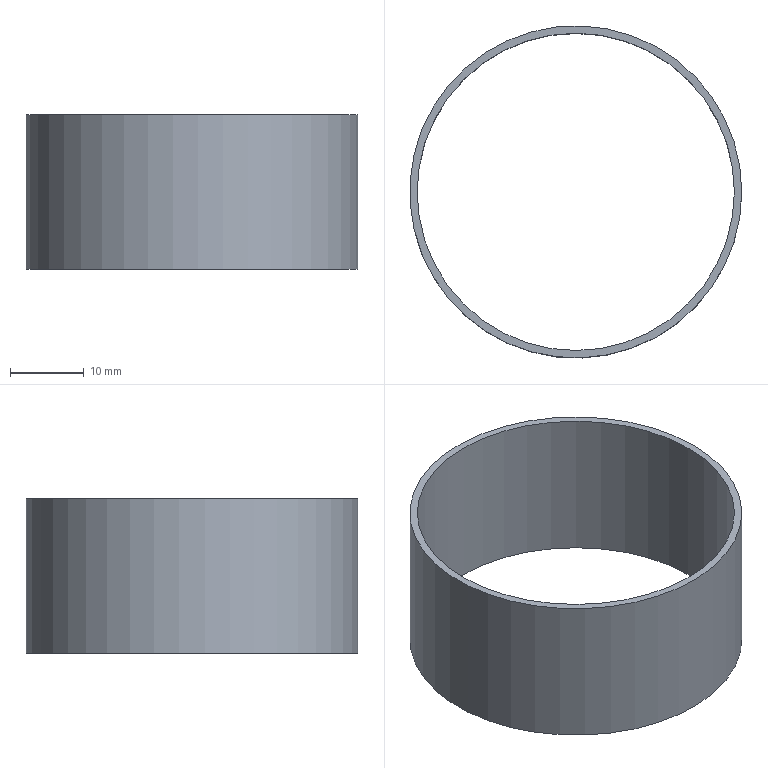Part | NX | features solid 2 | 1 solid | 4 faces | box 45 x 45 x 21 mm | volume 2903 mm3 | cylinder 2 | plane 2 | commonest cylinder face diameters 43 x1 45 x1
STEP:
#1=CARTESIAN_POINT('',(537.719,189.417,21.));
#2=VERTEX_POINT('',#1);
#3=CARTESIAN_POINT('',(515.219,189.417,21.));
#4=DIRECTION('',(0.,0.,1.));
#5=DIRECTION('',(1.,0.,0.));
#6=AXIS2_PLACEMENT_3D('',#3,#4,#5);
#7=CIRCLE('',#6,22.5);
#8=EDGE_CURVE('',#2,#2,#7,.T.);
#9=ORIENTED_EDGE('',*,*,#8,.F.);
#10=EDGE_LOOP('',(#9));
#11=FACE_BOUND('',#10,.T.);
#12=CARTESIAN_POINT('',(537.719,189.417,0.));
#13=VERTEX_POINT('',#12);
#14=CARTESIAN_POINT('',(515.219,189.417,0.));
#15=DIRECTION('',(0.,0.,1.));
#16=DIRECTION('',(1.,0.,0.));
#17=AXIS2_PLACEMENT_3D('',#14,#15,#16);
#18=CIRCLE('',#17,22.5);
#19=EDGE_CURVE('',#13,#13,#18,.T.);
#20=ORIENTED_EDGE('',*,*,#19,.T.);
#21=EDGE_LOOP('',(#20));
#22=FACE_BOUND('',#21,.T.);
#23=CARTESIAN_POINT('',(515.219,189.417,21.));
#24=DIRECTION('',(0.,0.,-1.));
#25=DIRECTION('',(-1.,0.,0.));
#26=AXIS2_PLACEMENT_3D('',#23,#24,#25);
#27=CYLINDRICAL_SURFACE('',#26,22.5);
#28=ADVANCED_FACE('',(#11,#22),#27,.T.);
#29=CARTESIAN_POINT('',(536.719,189.417,21.));
#30=VERTEX_POINT('',#29);
#31=CARTESIAN_POINT('',(515.219,189.417,21.));
#32=DIRECTION('',(0.,0.,1.));
#33=DIRECTION('',(1.,0.,0.));
#34=AXIS2_PLACEMENT_3D('',#31,#32,#33);
#35=CIRCLE('',#34,21.5);
#36=EDGE_CURVE('',#30,#30,#35,.T.);
#37=ORIENTED_EDGE('',*,*,#36,.T.);
#38=EDGE_LOOP('',(#37));
#39=FACE_BOUND('',#38,.T.);
#40=CARTESIAN_POINT('',(536.719,189.417,0.));
#41=VERTEX_POINT('',#40);
#42=CARTESIAN_POINT('',(515.219,189.417,0.));
#43=DIRECTION('',(0.,0.,1.));
#44=DIRECTION('',(1.,0.,0.));
#45=AXIS2_PLACEMENT_3D('',#42,#43,#44);
#46=CIRCLE('',#45,21.5);
#47=EDGE_CURVE('',#41,#41,#46,.T.);
#48=ORIENTED_EDGE('',*,*,#47,.F.);
#49=EDGE_LOOP('',(#48));
#50=FACE_BOUND('',#49,.T.);
#51=CARTESIAN_POINT('',(515.219,189.417,21.));
#52=DIRECTION('',(0.,0.,-1.));
#53=DIRECTION('',(-1.,0.,0.));
#54=AXIS2_PLACEMENT_3D('',#51,#52,#53);
#55=CYLINDRICAL_SURFACE('',#54,21.5);
#56=ADVANCED_FACE('',(#39,#50),#55,.F.);
#57=ORIENTED_EDGE('',*,*,#8,.T.);
#58=EDGE_LOOP('',(#57));
#59=FACE_BOUND('',#58,.T.);
#60=ORIENTED_EDGE('',*,*,#36,.F.);
#61=EDGE_LOOP('',(#60));
#62=FACE_BOUND('',#61,.T.);
#63=CARTESIAN_POINT('',(515.219,189.417,21.));
#64=DIRECTION('',(0.,0.,1.));
#65=DIRECTION('',(1.,0.,0.));
#66=AXIS2_PLACEMENT_3D('',#63,#64,#65);
#67=PLANE('',#66);
#68=ADVANCED_FACE('',(#59,#62),#67,.T.);
#69=ORIENTED_EDGE('',*,*,#19,.F.);
#70=EDGE_LOOP('',(#69));
#71=FACE_BOUND('',#70,.T.);
#72=ORIENTED_EDGE('',*,*,#47,.T.);
#73=EDGE_LOOP('',(#72));
#74=FACE_BOUND('',#73,.T.);
#75=CARTESIAN_POINT('',(515.219,189.417,0.));
#76=DIRECTION('',(0.,0.,1.));
#77=DIRECTION('',(1.,0.,0.));
#78=AXIS2_PLACEMENT_3D('',#75,#76,#77);
#79=PLANE('',#78);
#80=ADVANCED_FACE('',(#71,#74),#79,.F.);
#81=CLOSED_SHELL('',(#28,#56,#68,#80));
#82=MANIFOLD_SOLID_BREP('',#81);
#83=(LENGTH_UNIT()NAMED_UNIT(*)SI_UNIT(.MILLI.,.METRE.));
#84=UNCERTAINTY_MEASURE_WITH_UNIT(LENGTH_MEASURE(0.00001),#83,'','');
#85=(NAMED_UNIT(*)PLANE_ANGLE_UNIT()SI_UNIT($,.RADIAN.));
#86=(NAMED_UNIT(*)SI_UNIT($,.STERADIAN.)SOLID_ANGLE_UNIT());
#87=(GEOMETRIC_REPRESENTATION_CONTEXT(3)GLOBAL_UNCERTAINTY_ASSIGNED_CONTEXT((#84))GLOBAL_UNIT_ASSIGNED_CONTEXT((#83,#85,#86))REPRESENTATION_CONTEXT('',''));
#88=ADVANCED_BREP_SHAPE_REPRESENTATION('',(#82),#87);